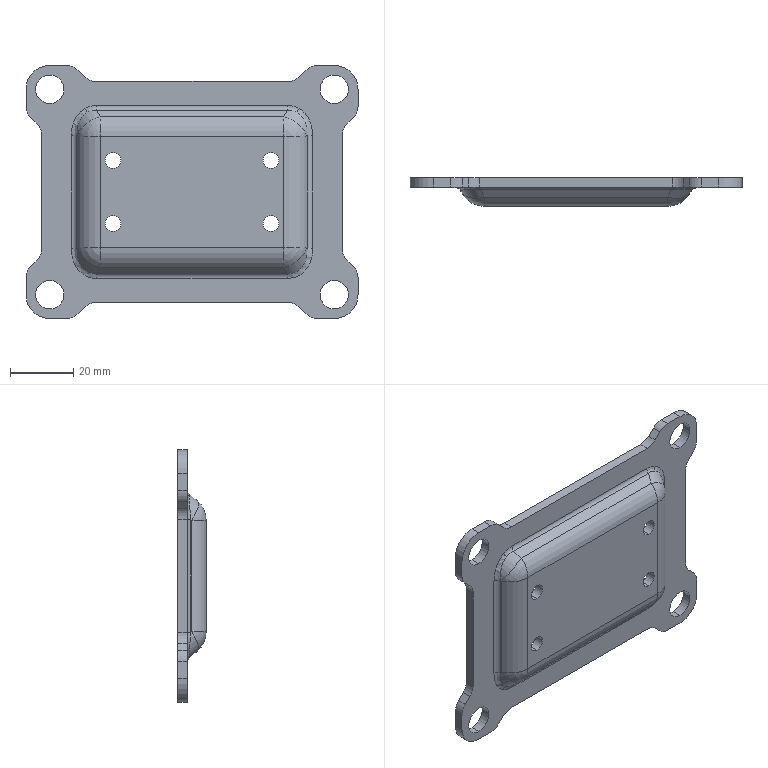Part | SolidWorks | features ICE 3, MirrorPattern 3, CornerTrim 2, FlatPattern 1, FormToolInstance 1, HoleWzd 1, SMBaseFlange 1, SheetMetal 1 | 1 solid | 112 faces | box 105 x 9 x 80 mm | volume 22120 mm3 | cylinder 60 | plane 32 | spline 12 | sphere 8 | commonest cylinder face diameters 10 x28 5 x8 9 x8 16 x8 4 x4 15 x4